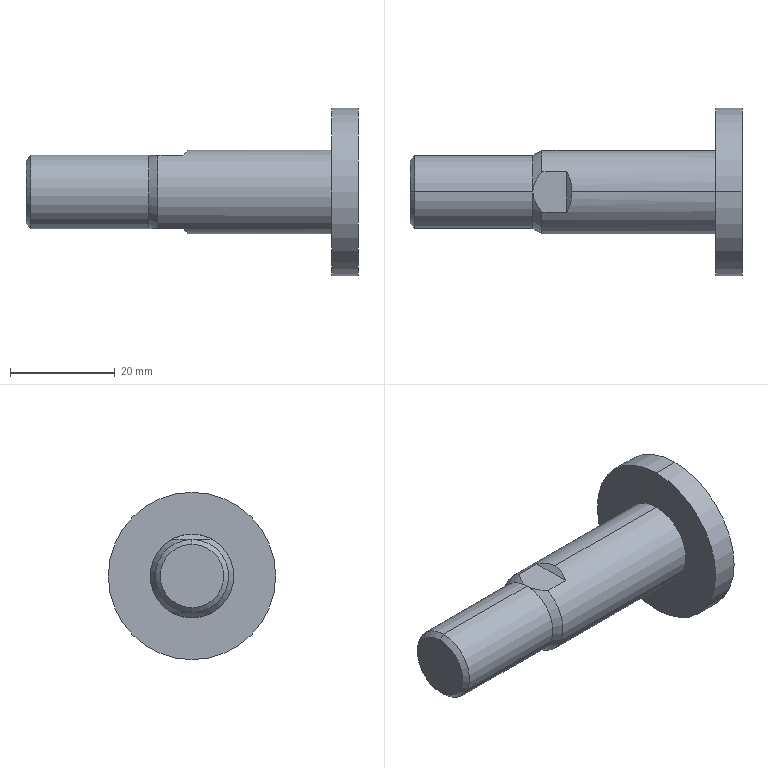Part | STEP file | SceondHI_CDQ2B32-20CMA93(0_0)_CYROD_Default | 1 solid | 17 faces | box 63.5 x 32 x 32 mm | volume 14555 mm3 | plane 7 | cylinder 6 | cone 4 | commonest cylinder face diameters 14 x2 16 x2 32 x2
STEP:
#1=CARTESIAN_POINT('',(0.,0.,0.));
#2=DIRECTION('',(0.,0.,1.));
#3=DIRECTION('',(1.,0.,0.));
#4=AXIS2_PLACEMENT_3D('',#1,#2,#3);
#5=CARTESIAN_POINT('',(30.,0.,8.));
#6=VERTEX_POINT('',#5);
#7=CARTESIAN_POINT('',(30.,0.,-8.));
#8=VERTEX_POINT('',#7);
#9=CARTESIAN_POINT('',(30.,0.,0.));
#10=DIRECTION('',(-1.,0.,0.));
#11=DIRECTION('',(0.,0.,1.));
#12=AXIS2_PLACEMENT_3D('',#9,#10,#11);
#13=CIRCLE('',#12,8.);
#14=CARTESIAN_POINT('',(35.,0.,0.));
#15=DIRECTION('',(-1.,0.,0.));
#16=DIRECTION('',(0.,0.,1.));
#17=AXIS2_PLACEMENT_3D('',#14,#15,#16);
#18=CYLINDRICAL_SURFACE('',#17,8.);
#19=CARTESIAN_POINT('',(0.,5.));
#20=DIRECTION('',(1.,0.));
#21=VECTOR('',#20,1.);
#22=LINE('',#19,#21);
#23=(GEOMETRIC_REPRESENTATION_CONTEXT(2)PARAMETRIC_REPRESENTATION_CONTEXT()REPRESENTATION_CONTEXT('',''));
#24=DEFINITIONAL_REPRESENTATION('',(#22),#23);
#25=PCURVE('',#18,#24);
#26=CARTESIAN_POINT('',(30.,8.,0.));
#27=DIRECTION('',(1.,0.,0.));
#28=DIRECTION('',(0.,0.,-1.));
#29=AXIS2_PLACEMENT_3D('',#26,#27,#28);
#30=PLANE('',#29);
#31=CARTESIAN_POINT('',(-8.,-8.));
#32=CARTESIAN_POINT('',(-8.,5.856));
#33=CARTESIAN_POINT('',(4.,-1.072));
#34=CARTESIAN_POINT('',(16.,-8.));
#35=CARTESIAN_POINT('',(4.,-14.928));
#36=CARTESIAN_POINT('',(-8.,-21.856));
#37=CARTESIAN_POINT('',(-8.,-8.));
#38=(BOUNDED_CURVE()B_SPLINE_CURVE(2,(#31,#32,#33,#34,#35,#36,#37),.UNSPECIFIED.,.T.,.F.)B_SPLINE_CURVE_WITH_KNOTS((1,2,2,2,2,1),(-2.094,0.,2.094,4.189,6.283,8.378),.UNSPECIFIED.)CURVE()GEOMETRIC_REPRESENTATION_ITEM()RATIONAL_B_SPLINE_CURVE((1.,0.5,1.,0.5,1.,0.5,1.))REPRESENTATION_ITEM(''));
#39=(GEOMETRIC_REPRESENTATION_CONTEXT(2)PARAMETRIC_REPRESENTATION_CONTEXT()REPRESENTATION_CONTEXT('',''));
#40=DEFINITIONAL_REPRESENTATION('',(#38),#39);
#41=PCURVE('',#30,#40);
#42=SURFACE_CURVE('',#13,(#25,#41),.PCURVE_S1.);
#43=EDGE_CURVE('',#6,#8,#42,.T.);
#44=ORIENTED_EDGE('',*,*,#43,.T.);
#45=CARTESIAN_POINT('',(2.5,0.,-8.));
#46=VERTEX_POINT('',#45);
#47=CARTESIAN_POINT('',(35.,0.,-8.));
#48=DIRECTION('',(-1.,0.,0.));
#49=VECTOR('',#48,1.);
#50=LINE('',#47,#49);
#51=CARTESIAN_POINT('',(3.142,0.));
#52=DIRECTION('',(0.,1.));
#53=VECTOR('',#52,1.);
#54=LINE('',#51,#53);
#55=(GEOMETRIC_REPRESENTATION_CONTEXT(2)PARAMETRIC_REPRESENTATION_CONTEXT()REPRESENTATION_CONTEXT('',''));
#56=DEFINITIONAL_REPRESENTATION('',(#54),#55);
#57=PCURVE('',#18,#56);
#58=CARTESIAN_POINT('',(35.,0.,0.));
#59=DIRECTION('',(-1.,0.,0.));
#60=DIRECTION('',(0.,0.,1.));
#61=AXIS2_PLACEMENT_3D('',#58,#59,#60);
#62=CYLINDRICAL_SURFACE('',#61,8.);
#63=CARTESIAN_POINT('',(3.142,0.));
#64=DIRECTION('',(0.,1.));
#65=VECTOR('',#64,1.);
#66=LINE('',#63,#65);
#67=(GEOMETRIC_REPRESENTATION_CONTEXT(2)PARAMETRIC_REPRESENTATION_CONTEXT()REPRESENTATION_CONTEXT('',''));
#68=DEFINITIONAL_REPRESENTATION('',(#66),#67);
#69=PCURVE('',#62,#68);
#70=SURFACE_CURVE('',#50,(#57,#69),.PCURVE_S1.);
#71=EDGE_CURVE('',#8,#46,#70,.T.);
#72=ORIENTED_EDGE('',*,*,#71,.T.);
#73=CARTESIAN_POINT('',(1.5,3.873,-7.));
#74=VERTEX_POINT('',#73);
#75=CARTESIAN_POINT('',(2.5,0.,-8.));
#76=CARTESIAN_POINT('',(2.5,1.362,-8.));
#77=CARTESIAN_POINT('',(2.159,2.681,-7.659));
#78=CARTESIAN_POINT('',(1.5,3.873,-7.));
#79=(BOUNDED_CURVE()B_SPLINE_CURVE(3,(#75,#76,#77,#78),.UNSPECIFIED.,.F.,.F.)B_SPLINE_CURVE_WITH_KNOTS((4,4),(3.142,3.647),.PIECEWISE_BEZIER_KNOTS.)CURVE()GEOMETRIC_REPRESENTATION_ITEM()RATIONAL_B_SPLINE_CURVE((1.,0.9788,0.9788,1.))REPRESENTATION_ITEM(''));
#80=CARTESIAN_POINT('',(3.142,32.5));
#81=CARTESIAN_POINT('',(3.134,32.5));
#82=CARTESIAN_POINT('',(3.119,32.501));
#83=CARTESIAN_POINT('',(3.096,32.508));
#84=CARTESIAN_POINT('',(3.073,32.518));
#85=CARTESIAN_POINT('',(3.05,32.533));
#86=CARTESIAN_POINT('',(3.027,32.552));
#87=CARTESIAN_POINT('',(3.004,32.575));
#88=CARTESIAN_POINT('',(2.981,32.602));
#89=CARTESIAN_POINT('',(2.958,32.634));
#90=CARTESIAN_POINT('',(2.935,32.669));
#91=CARTESIAN_POINT('',(2.912,32.709));
#92=CARTESIAN_POINT('',(2.889,32.753));
#93=CARTESIAN_POINT('',(2.866,32.802));
#94=CARTESIAN_POINT('',(2.843,32.854));
#95=CARTESIAN_POINT('',(2.82,32.91));
#96=CARTESIAN_POINT('',(2.797,32.971));
#97=CARTESIAN_POINT('',(2.774,33.035));
#98=CARTESIAN_POINT('',(2.751,33.103));
#99=CARTESIAN_POINT('',(2.728,33.175));
#100=CARTESIAN_POINT('',(2.705,33.251));
#101=CARTESIAN_POINT('',(2.682,33.33));
#102=CARTESIAN_POINT('',(2.659,33.413));
#103=CARTESIAN_POINT('',(2.644,33.471));
#104=CARTESIAN_POINT('',(2.636,33.5));
#105=B_SPLINE_CURVE_WITH_KNOTS('',3,(#80,#81,#82,#83,#84,#85,#86,#87,#88,#89,#90,#91,#92,#93,#94,#95,#96,#97,#98,#99,#100,#101,#102,#103,#104),.UNSPECIFIED.,.F.,.F.,(4,1,1,1,1,1,1,1,1,1,1,1,1,1,1,1,1,1,1,1,1,1,4),(3.142,3.165,3.188,3.211,3.233,3.256,3.279,3.302,3.325,3.348,3.371,3.394,3.417,3.44,3.463,3.486,3.509,3.532,3.555,3.578,3.601,3.624,3.647),.QUASI_UNIFORM_KNOTS.);
#106=(GEOMETRIC_REPRESENTATION_CONTEXT(2)PARAMETRIC_REPRESENTATION_CONTEXT()REPRESENTATION_CONTEXT('',''));
#107=DEFINITIONAL_REPRESENTATION('',(#105),#106);
#108=PCURVE('',#18,#107);
#109=CARTESIAN_POINT('',(1.5,16.,-7.));
#110=DIRECTION('',(-0.7071,0.,-0.7071));
#111=DIRECTION('',(-0.7071,0.,0.7071));
#112=AXIS2_PLACEMENT_3D('',#109,#110,#111);
#113=PLANE('',#112);
#114=CARTESIAN_POINT('',(-1.414,-16.));
#115=CARTESIAN_POINT('',(-1.414,-14.638));
#116=CARTESIAN_POINT('',(-0.9326,-13.319));
#117=CARTESIAN_POINT('',(0.,-12.127));
#118=(BOUNDED_CURVE()B_SPLINE_CURVE(3,(#114,#115,#116,#117),.UNSPECIFIED.,.F.,.F.)B_SPLINE_CURVE_WITH_KNOTS((4,4),(3.142,3.647),.PIECEWISE_BEZIER_KNOTS.)CURVE()GEOMETRIC_REPRESENTATION_ITEM()RATIONAL_B_SPLINE_CURVE((1.,0.9788,0.9788,1.))REPRESENTATION_ITEM(''));
#119=(GEOMETRIC_REPRESENTATION_CONTEXT(2)PARAMETRIC_REPRESENTATION_CONTEXT()REPRESENTATION_CONTEXT('',''));
#120=DEFINITIONAL_REPRESENTATION('',(#118),#119);
#121=PCURVE('',#113,#120);
#122=SURFACE_CURVE('',#79,(#108,#121),.PCURVE_S1.);
#123=EDGE_CURVE('',#46,#74,#122,.T.);
#124=ORIENTED_EDGE('',*,*,#123,.T.);
#125=CARTESIAN_POINT('',(-3.268,3.873,-7.));
#126=VERTEX_POINT('',#125);
#127=CARTESIAN_POINT('',(35.,3.873,-7.));
#128=DIRECTION('',(-1.,0.,0.));
#129=VECTOR('',#128,1.);
#130=LINE('',#127,#129);
#131=CARTESIAN_POINT('',(2.636,0.));
#132=DIRECTION('',(0.,1.));
#133=VECTOR('',#132,1.);
#134=LINE('',#131,#133);
#135=(GEOMETRIC_REPRESENTATION_CONTEXT(2)PARAMETRIC_REPRESENTATION_CONTEXT()REPRESENTATION_CONTEXT('',''));
#136=DEFINITIONAL_REPRESENTATION('',(#134),#135);
#137=PCURVE('',#18,#136);
#138=CARTESIAN_POINT('',(-5.,16.,-7.));
#139=DIRECTION('',(0.,0.,-1.));
#140=DIRECTION('',(-1.,0.,0.));
#141=AXIS2_PLACEMENT_3D('',#138,#139,#140);
#142=PLANE('',#141);
#143=CARTESIAN_POINT('',(-40.,-12.127));
#144=DIRECTION('',(1.,0.));
#145=VECTOR('',#144,1.);
#146=LINE('',#143,#145);
#147=(GEOMETRIC_REPRESENTATION_CONTEXT(2)PARAMETRIC_REPRESENTATION_CONTEXT()REPRESENTATION_CONTEXT('',''));
#148=DEFINITIONAL_REPRESENTATION('',(#146),#147);
#149=PCURVE('',#142,#148);
#150=SURFACE_CURVE('',#130,(#137,#149),.PCURVE_S1.);
#151=EDGE_CURVE('',#74,#126,#150,.T.);
#152=ORIENTED_EDGE('',*,*,#151,.T.);
#153=CARTESIAN_POINT('',(-3.268,3.873,7.));
#154=VERTEX_POINT('',#153);
#155=CARTESIAN_POINT('',(-3.268,0.,0.));
#156=DIRECTION('',(1.,0.,0.));
#157=DIRECTION('',(0.,0.,1.));
#158=AXIS2_PLACEMENT_3D('',#155,#156,#157);
#159=CIRCLE('',#158,8.);
#160=CARTESIAN_POINT('',(6.283,38.268));
#161=DIRECTION('',(-1.,0.));
#162=VECTOR('',#161,1.);
#163=LINE('',#160,#162);
#164=(GEOMETRIC_REPRESENTATION_CONTEXT(2)PARAMETRIC_REPRESENTATION_CONTEXT()REPRESENTATION_CONTEXT('',''));
#165=DEFINITIONAL_REPRESENTATION('',(#163),#164);
#166=PCURVE('',#18,#165);
#167=CARTESIAN_POINT('',(-3.268,0.,0.));
#168=DIRECTION('',(1.,0.,0.));
#169=DIRECTION('',(0.,0.,-1.));
#170=AXIS2_PLACEMENT_3D('',#167,#168,#169);
#171=CONICAL_SURFACE('',#170,8.,0.5236);
#172=CARTESIAN_POINT('',(-3.142,0.));
#173=DIRECTION('',(1.,0.));
#174=VECTOR('',#173,1.);
#175=LINE('',#172,#174);
#176=(GEOMETRIC_REPRESENTATION_CONTEXT(2)PARAMETRIC_REPRESENTATION_CONTEXT()REPRESENTATION_CONTEXT('',''));
#177=DEFINITIONAL_REPRESENTATION('',(#175),#176);
#178=PCURVE('',#171,#177);
#179=SURFACE_CURVE('',#159,(#166,#178),.PCURVE_S1.);
#180=EDGE_CURVE('',#126,#154,#179,.T.);
#181=ORIENTED_EDGE('',*,*,#180,.T.);
#182=CARTESIAN_POINT('',(1.5,3.873,7.));
#183=VERTEX_POINT('',#182);
#184=CARTESIAN_POINT('',(35.,3.873,7.));
#185=DIRECTION('',(1.,0.,0.));
#186=VECTOR('',#185,1.);
#187=LINE('',#184,#186);
#188=CARTESIAN_POINT('',(0.5054,0.));
#189=DIRECTION('',(0.,-1.));
#190=VECTOR('',#189,1.);
#191=LINE('',#188,#190);
#192=(GEOMETRIC_REPRESENTATION_CONTEXT(2)PARAMETRIC_REPRESENTATION_CONTEXT()REPRESENTATION_CONTEXT('',''));
#193=DEFINITIONAL_REPRESENTATION('',(#191),#192);
#194=PCURVE('',#18,#193);
#195=CARTESIAN_POINT('',(1.5,16.,7.));
#196=DIRECTION('',(0.,0.,1.));
#197=DIRECTION('',(1.,0.,0.));
#198=AXIS2_PLACEMENT_3D('',#195,#196,#197);
#199=PLANE('',#198);
#200=CARTESIAN_POINT('',(33.5,-12.127));
#201=DIRECTION('',(1.,0.));
#202=VECTOR('',#201,1.);
#203=LINE('',#200,#202);
#204=(GEOMETRIC_REPRESENTATION_CONTEXT(2)PARAMETRIC_REPRESENTATION_CONTEXT()REPRESENTATION_CONTEXT('',''));
#205=DEFINITIONAL_REPRESENTATION('',(#203),#204);
#206=PCURVE('',#199,#205);
#207=SURFACE_CURVE('',#187,(#194,#206),.PCURVE_S1.);
#208=EDGE_CURVE('',#154,#183,#207,.T.);
#209=ORIENTED_EDGE('',*,*,#208,.T.);
#210=CARTESIAN_POINT('',(2.5,0.,8.));
#211=VERTEX_POINT('',#210);
#212=CARTESIAN_POINT('',(1.5,3.873,7.));
#213=CARTESIAN_POINT('',(2.159,2.681,7.659));
#214=CARTESIAN_POINT('',(2.5,1.362,8.));
#215=CARTESIAN_POINT('',(2.5,0.,8.));
#216=(BOUNDED_CURVE()B_SPLINE_CURVE(3,(#212,#213,#214,#215),.UNSPECIFIED.,.F.,.F.)B_SPLINE_CURVE_WITH_KNOTS((4,4),(2.636,3.142),.PIECEWISE_BEZIER_KNOTS.)CURVE()GEOMETRIC_REPRESENTATION_ITEM()RATIONAL_B_SPLINE_CURVE((1.,0.9788,0.9788,1.))REPRESENTATION_ITEM(''));
#217=CARTESIAN_POINT('',(0.5054,33.5));
#218=CARTESIAN_POINT('',(0.4978,33.471));
#219=CARTESIAN_POINT('',(0.4826,33.413));
#220=CARTESIAN_POINT('',(0.4598,33.33));
#221=CARTESIAN_POINT('',(0.4369,33.251));
#222=CARTESIAN_POINT('',(0.414,33.175));
#223=CARTESIAN_POINT('',(0.391,33.103));
#224=CARTESIAN_POINT('',(0.368,33.035));
#225=CARTESIAN_POINT('',(0.345,32.971));
#226=CARTESIAN_POINT('',(0.3219,32.91));
#227=CARTESIAN_POINT('',(0.2989,32.854));
#228=CARTESIAN_POINT('',(0.2758,32.802));
#229=CARTESIAN_POINT('',(0.2527,32.753));
#230=CARTESIAN_POINT('',(0.2296,32.709));
#231=CARTESIAN_POINT('',(0.2065,32.669));
#232=CARTESIAN_POINT('',(0.1834,32.634));
#233=CARTESIAN_POINT('',(0.1604,32.602));
#234=CARTESIAN_POINT('',(0.1373,32.575));
#235=CARTESIAN_POINT('',(0.1143,32.552));
#236=CARTESIAN_POINT('',(0.09137,32.533));
#237=CARTESIAN_POINT('',(0.06844,32.518));
#238=CARTESIAN_POINT('',(0.04557,32.508));
#239=CARTESIAN_POINT('',(0.02275,32.501));
#240=CARTESIAN_POINT('',(0.007576,32.5));
#241=CARTESIAN_POINT('',(0.,32.5));
#242=B_SPLINE_CURVE_WITH_KNOTS('',3,(#217,#218,#219,#220,#221,#222,#223,#224,#225,#226,#227,#228,#229,#230,#231,#232,#233,#234,#235,#236,#237,#238,#239,#240,#241),.UNSPECIFIED.,.F.,.F.,(4,1,1,1,1,1,1,1,1,1,1,1,1,1,1,1,1,1,1,1,1,1,4),(2.636,2.659,2.682,2.705,2.728,2.751,2.774,2.797,2.82,2.843,2.866,2.889,2.912,2.935,2.958,2.981,3.004,3.027,3.05,3.073,3.096,3.119,3.142),.QUASI_UNIFORM_KNOTS.);
#243=(GEOMETRIC_REPRESENTATION_CONTEXT(2)PARAMETRIC_REPRESENTATION_CONTEXT()REPRESENTATION_CONTEXT('',''));
#244=DEFINITIONAL_REPRESENTATION('',(#242),#243);
#245=PCURVE('',#18,#244);
#246=CARTESIAN_POINT('',(6.5,16.,12.));
#247=DIRECTION('',(-0.7071,0.,0.7071));
#248=DIRECTION('',(0.7071,0.,0.7071));
#249=AXIS2_PLACEMENT_3D('',#246,#247,#248);
#250=PLANE('',#249);
#251=CARTESIAN_POINT('',(-7.071,-12.127));
#252=CARTESIAN_POINT('',(-6.138,-13.319));
#253=CARTESIAN_POINT('',(-5.657,-14.638));
#254=CARTESIAN_POINT('',(-5.657,-16.));
#255=(BOUNDED_CURVE()B_SPLINE_CURVE(3,(#251,#252,#253,#254),.UNSPECIFIED.,.F.,.F.)B_SPLINE_CURVE_WITH_KNOTS((4,4),(2.636,3.142),.PIECEWISE_BEZIER_KNOTS.)CURVE()GEOMETRIC_REPRESENTATION_ITEM()RATIONAL_B_SPLINE_CURVE((1.,0.9788,0.9788,1.))REPRESENTATION_ITEM(''));
#256=(GEOMETRIC_REPRESENTATION_CONTEXT(2)PARAMETRIC_REPRESENTATION_CONTEXT()REPRESENTATION_CONTEXT('',''));
#257=DEFINITIONAL_REPRESENTATION('',(#255),#256);
#258=PCURVE('',#250,#257);
#259=SURFACE_CURVE('',#216,(#245,#258),.PCURVE_S1.);
#260=EDGE_CURVE('',#183,#211,#259,.T.);
#261=ORIENTED_EDGE('',*,*,#260,.T.);
#262=CARTESIAN_POINT('',(35.,0.,8.));
#263=DIRECTION('',(-1.,0.,0.));
#264=VECTOR('',#263,1.);
#265=LINE('',#262,#264);
#266=CARTESIAN_POINT('',(0.,0.));
#267=DIRECTION('',(0.,1.));
#268=VECTOR('',#267,1.);
#269=LINE('',#266,#268);
#270=(GEOMETRIC_REPRESENTATION_CONTEXT(2)PARAMETRIC_REPRESENTATION_CONTEXT()REPRESENTATION_CONTEXT('',''));
#271=DEFINITIONAL_REPRESENTATION('',(#269),#270);
#272=PCURVE('',#18,#271);
#273=CARTESIAN_POINT('',(6.283,0.));
#274=DIRECTION('',(0.,1.));
#275=VECTOR('',#274,1.);
#276=LINE('',#273,#275);
#277=(GEOMETRIC_REPRESENTATION_CONTEXT(2)PARAMETRIC_REPRESENTATION_CONTEXT()REPRESENTATION_CONTEXT('',''));
#278=DEFINITIONAL_REPRESENTATION('',(#276),#277);
#279=PCURVE('',#62,#278);
#280=SURFACE_CURVE('',#265,(#272,#279),.PCURVE_S1.);
#281=EDGE_CURVE('',#6,#211,#280,.T.);
#282=ORIENTED_EDGE('',*,*,#281,.F.);
#283=EDGE_LOOP('',(#44,#72,#124,#152,#181,#209,#261,#282));
#284=FACE_BOUND('',#283,.T.);
#285=ADVANCED_FACE('',(#284),#18,.T.);
#286=CARTESIAN_POINT('',(-5.,0.,-7.));
#287=VERTEX_POINT('',#286);
#288=CARTESIAN_POINT('',(-5.,0.,7.));
#289=VERTEX_POINT('',#288);
#290=CARTESIAN_POINT('',(-5.,0.,0.));
#291=DIRECTION('',(1.,0.,0.));
#292=DIRECTION('',(0.,0.,-1.));
#293=AXIS2_PLACEMENT_3D('',#290,#291,#292);
#294=CIRCLE('',#293,7.);
#295=CARTESIAN_POINT('',(35.,0.,0.));
#296=DIRECTION('',(-1.,0.,0.));
#297=DIRECTION('',(0.,0.,1.));
#298=AXIS2_PLACEMENT_3D('',#295,#296,#297);
#299=CYLINDRICAL_SURFACE('',#298,7.);
#300=CARTESIAN_POINT('',(3.142,40.));
#301=DIRECTION('',(-1.,0.));
#302=VECTOR('',#301,1.);
#303=LINE('',#300,#302);
#304=(GEOMETRIC_REPRESENTATION_CONTEXT(2)PARAMETRIC_REPRESENTATION_CONTEXT()REPRESENTATION_CONTEXT('',''));
#305=DEFINITIONAL_REPRESENTATION('',(#303),#304);
#306=PCURVE('',#299,#305);
#307=CARTESIAN_POINT('',(0.,-1.732));
#308=DIRECTION('',(1.,0.));
#309=VECTOR('',#308,1.);
#310=LINE('',#307,#309);
#311=(GEOMETRIC_REPRESENTATION_CONTEXT(2)PARAMETRIC_REPRESENTATION_CONTEXT()REPRESENTATION_CONTEXT('',''));
#312=DEFINITIONAL_REPRESENTATION('',(#310),#311);
#313=PCURVE('',#171,#312);
#314=SURFACE_CURVE('',#294,(#306,#313),.PCURVE_S1.);
#315=EDGE_CURVE('',#287,#289,#314,.T.);
#316=ORIENTED_EDGE('',*,*,#315,.F.);
#317=CARTESIAN_POINT('',(-27.58,0.,-7.));
#318=VERTEX_POINT('',#317);
#319=CARTESIAN_POINT('',(35.,0.,-7.));
#320=DIRECTION('',(-1.,0.,0.));
#321=VECTOR('',#320,1.);
#322=LINE('',#319,#321);
#323=CARTESIAN_POINT('',(3.142,0.));
#324=DIRECTION('',(0.,1.));
#325=VECTOR('',#324,1.);
#326=LINE('',#323,#325);
#327=(GEOMETRIC_REPRESENTATION_CONTEXT(2)PARAMETRIC_REPRESENTATION_CONTEXT()REPRESENTATION_CONTEXT('',''));
#328=DEFINITIONAL_REPRESENTATION('',(#326),#327);
#329=PCURVE('',#299,#328);
#330=CARTESIAN_POINT('',(35.,0.,0.));
#331=DIRECTION('',(-1.,0.,0.));
#332=DIRECTION('',(0.,0.,1.));
#333=AXIS2_PLACEMENT_3D('',#330,#331,#332);
#334=CYLINDRICAL_SURFACE('',#333,7.);
#335=CARTESIAN_POINT('',(3.142,0.));
#336=DIRECTION('',(0.,1.));
#337=VECTOR('',#336,1.);
#338=LINE('',#335,#337);
#339=(GEOMETRIC_REPRESENTATION_CONTEXT(2)PARAMETRIC_REPRESENTATION_CONTEXT()REPRESENTATION_CONTEXT('',''));
#340=DEFINITIONAL_REPRESENTATION('',(#338),#339);
#341=PCURVE('',#334,#340);
#342=SURFACE_CURVE('',#322,(#329,#341),.PCURVE_S1.);
#343=EDGE_CURVE('',#287,#318,#342,.T.);
#344=ORIENTED_EDGE('',*,*,#343,.T.);
#345=CARTESIAN_POINT('',(-27.58,0.,7.));
#346=VERTEX_POINT('',#345);
#347=CARTESIAN_POINT('',(-27.58,0.,0.));
#348=DIRECTION('',(1.,0.,0.));
#349=DIRECTION('',(0.,0.,1.));
#350=AXIS2_PLACEMENT_3D('',#347,#348,#349);
#351=CIRCLE('',#350,7.);
#352=CARTESIAN_POINT('',(6.283,62.58));
#353=DIRECTION('',(-1.,0.));
#354=VECTOR('',#353,1.);
#355=LINE('',#352,#354);
#356=(GEOMETRIC_REPRESENTATION_CONTEXT(2)PARAMETRIC_REPRESENTATION_CONTEXT()REPRESENTATION_CONTEXT('',''));
#357=DEFINITIONAL_REPRESENTATION('',(#355),#356);
#358=PCURVE('',#299,#357);
#359=CARTESIAN_POINT('',(-27.58,0.,0.));
#360=DIRECTION('',(1.,0.,0.));
#361=DIRECTION('',(0.,0.,-1.));
#362=AXIS2_PLACEMENT_3D('',#359,#360,#361);
#363=CONICAL_SURFACE('',#362,7.,0.7854);
#364=CARTESIAN_POINT('',(-3.142,0.));
#365=DIRECTION('',(1.,0.));
#366=VECTOR('',#365,1.);
#367=LINE('',#364,#366);
#368=(GEOMETRIC_REPRESENTATION_CONTEXT(2)PARAMETRIC_REPRESENTATION_CONTEXT()REPRESENTATION_CONTEXT('',''));
#369=DEFINITIONAL_REPRESENTATION('',(#367),#368);
#370=PCURVE('',#363,#369);
#371=SURFACE_CURVE('',#351,(#358,#370),.PCURVE_S1.);
#372=EDGE_CURVE('',#318,#346,#371,.T.);
#373=ORIENTED_EDGE('',*,*,#372,.T.);
#374=CARTESIAN_POINT('',(35.,0.,7.));
#375=DIRECTION('',(-1.,0.,0.));
#376=VECTOR('',#375,1.);
#377=LINE('',#374,#376);
#378=CARTESIAN_POINT('',(0.,0.));
#379=DIRECTION('',(0.,1.));
#380=VECTOR('',#379,1.);
#381=LINE('',#378,#380);
#382=(GEOMETRIC_REPRESENTATION_CONTEXT(2)PARAMETRIC_REPRESENTATION_CONTEXT()REPRESENTATION_CONTEXT('',''));
#383=DEFINITIONAL_REPRESENTATION('',(#381),#382);
#384=PCURVE('',#299,#383);
#385=CARTESIAN_POINT('',(6.283,0.));
#386=DIRECTION('',(0.,1.));
#387=VECTOR('',#386,1.);
#388=LINE('',#385,#387);
#389=(GEOMETRIC_REPRESENTATION_CONTEXT(2)PARAMETRIC_REPRESENTATION_CONTEXT()REPRESENTATION_CONTEXT('',''));
#390=DEFINITIONAL_REPRESENTATION('',(#388),#389);
#391=PCURVE('',#334,#390);
#392=SURFACE_CURVE('',#377,(#384,#391),.PCURVE_S1.);
#393=EDGE_CURVE('',#289,#346,#392,.T.);
#394=ORIENTED_EDGE('',*,*,#393,.F.);
#395=EDGE_LOOP('',(#316,#344,#373,#394));
#396=FACE_BOUND('',#395,.T.);
#397=ADVANCED_FACE('',(#396),#299,.T.);
#398=CARTESIAN_POINT('',(35.,0.,16.));
#399=VERTEX_POINT('',#398);
#400=CARTESIAN_POINT('',(35.,0.,-16.));
#401=VERTEX_POINT('',#400);
#402=CARTESIAN_POINT('',(35.,0.,0.));
#403=DIRECTION('',(-1.,0.,0.));
#404=DIRECTION('',(0.,0.,1.));
#405=AXIS2_PLACEMENT_3D('',#402,#403,#404);
#406=CIRCLE('',#405,16.);
#407=CARTESIAN_POINT('',(35.,0.,0.));
#408=DIRECTION('',(-1.,0.,0.));
#409=DIRECTION('',(0.,0.,1.));
#410=AXIS2_PLACEMENT_3D('',#407,#408,#409);
#411=CYLINDRICAL_SURFACE('',#410,16.);
#412=CARTESIAN_POINT('',(0.,0.));
#413=DIRECTION('',(1.,0.));
#414=VECTOR('',#413,1.);
#415=LINE('',#412,#414);
#416=(GEOMETRIC_REPRESENTATION_CONTEXT(2)PARAMETRIC_REPRESENTATION_CONTEXT()REPRESENTATION_CONTEXT('',''));
#417=DEFINITIONAL_REPRESENTATION('',(#415),#416);
#418=PCURVE('',#411,#417);
#419=CARTESIAN_POINT('',(35.,16.,0.));
#420=DIRECTION('',(-1.,0.,0.));
#421=DIRECTION('',(0.,0.,1.));
#422=AXIS2_PLACEMENT_3D('',#419,#420,#421);
#423=PLANE('',#422);
#424=CARTESIAN_POINT('',(0.,-16.));
#425=DIRECTION('',(1.,0.));
#426=AXIS2_PLACEMENT_2D('',#424,#425);
#427=CIRCLE('',#426,16.);
#428=(GEOMETRIC_REPRESENTATION_CONTEXT(2)PARAMETRIC_REPRESENTATION_CONTEXT()REPRESENTATION_CONTEXT('',''));
#429=DEFINITIONAL_REPRESENTATION('',(#427),#428);
#430=PCURVE('',#423,#429);
#431=SURFACE_CURVE('',#406,(#418,#430),.PCURVE_S1.);
#432=EDGE_CURVE('',#399,#401,#431,.T.);
#433=ORIENTED_EDGE('',*,*,#432,.T.);
#434=CARTESIAN_POINT('',(30.,0.,-16.));
#435=VERTEX_POINT('',#434);
#436=CARTESIAN_POINT('',(35.,0.,-16.));
#437=DIRECTION('',(-1.,0.,0.));
#438=VECTOR('',#437,1.);
#439=LINE('',#436,#438);
#440=CARTESIAN_POINT('',(3.142,0.));
#441=DIRECTION('',(0.,1.));
#442=VECTOR('',#441,1.);
#443=LINE('',#440,#442);
#444=(GEOMETRIC_REPRESENTATION_CONTEXT(2)PARAMETRIC_REPRESENTATION_CONTEXT()REPRESENTATION_CONTEXT('',''));
#445=DEFINITIONAL_REPRESENTATION('',(#443),#444);
#446=PCURVE('',#411,#445);
#447=CARTESIAN_POINT('',(35.,0.,0.));
#448=DIRECTION('',(-1.,0.,0.));
#449=DIRECTION('',(0.,0.,1.));
#450=AXIS2_PLACEMENT_3D('',#447,#448,#449);
#451=CYLINDRICAL_SURFACE('',#450,16.);
#452=CARTESIAN_POINT('',(3.142,0.));
#453=DIRECTION('',(0.,1.));
#454=VECTOR('',#453,1.);
#455=LINE('',#452,#454);
#456=(GEOMETRIC_REPRESENTATION_CONTEXT(2)PARAMETRIC_REPRESENTATION_CONTEXT()REPRESENTATION_CONTEXT('',''));
#457=DEFINITIONAL_REPRESENTATION('',(#455),#456);
#458=PCURVE('',#451,#457);
#459=SURFACE_CURVE('',#439,(#446,#458),.PCURVE_S1.);
#460=EDGE_CURVE('',#401,#435,#459,.T.);
#461=ORIENTED_EDGE('',*,*,#460,.T.);
#462=CARTESIAN_POINT('',(30.,0.,16.));
#463=VERTEX_POINT('',#462);
#464=CARTESIAN_POINT('',(30.,0.,0.));
#465=DIRECTION('',(1.,0.,0.));
#466=DIRECTION('',(0.,0.,1.));
#467=AXIS2_PLACEMENT_3D('',#464,#465,#466);
#468=CIRCLE('',#467,16.);
#469=CARTESIAN_POINT('',(6.283,5.));
#470=DIRECTION('',(-1.,0.));
#471=VECTOR('',#470,1.);
#472=LINE('',#469,#471);
#473=(GEOMETRIC_REPRESENTATION_CONTEXT(2)PARAMETRIC_REPRESENTATION_CONTEXT()REPRESENTATION_CONTEXT('',''));
#474=DEFINITIONAL_REPRESENTATION('',(#472),#473);
#475=PCURVE('',#411,#474);
#476=CARTESIAN_POINT('',(0.,-8.));
#477=DIRECTION('',(-1.,0.));
#478=AXIS2_PLACEMENT_2D('',#476,#477);
#479=CIRCLE('',#478,16.);
#480=(GEOMETRIC_REPRESENTATION_CONTEXT(2)PARAMETRIC_REPRESENTATION_CONTEXT()REPRESENTATION_CONTEXT('',''));
#481=DEFINITIONAL_REPRESENTATION('',(#479),#480);
#482=PCURVE('',#30,#481);
#483=SURFACE_CURVE('',#468,(#475,#482),.PCURVE_S1.);
#484=EDGE_CURVE('',#435,#463,#483,.T.);
#485=ORIENTED_EDGE('',*,*,#484,.T.);
#486=CARTESIAN_POINT('',(35.,0.,16.));
#487=DIRECTION('',(-1.,0.,0.));
#488=VECTOR('',#487,1.);
#489=LINE('',#486,#488);
#490=CARTESIAN_POINT('',(0.,0.));
#491=DIRECTION('',(0.,1.));
#492=VECTOR('',#491,1.);
#493=LINE('',#490,#492);
#494=(GEOMETRIC_REPRESENTATION_CONTEXT(2)PARAMETRIC_REPRESENTATION_CONTEXT()REPRESENTATION_CONTEXT('',''));
#495=DEFINITIONAL_REPRESENTATION('',(#493),#494);
#496=PCURVE('',#411,#495);
#497=CARTESIAN_POINT('',(6.283,0.));
#498=DIRECTION('',(0.,1.));
#499=VECTOR('',#498,1.);
#500=LINE('',#497,#499);
#501=(GEOMETRIC_REPRESENTATION_CONTEXT(2)PARAMETRIC_REPRESENTATION_CONTEXT()REPRESENTATION_CONTEXT('',''));
#502=DEFINITIONAL_REPRESENTATION('',(#500),#501);
#503=PCURVE('',#451,#502);
#504=SURFACE_CURVE('',#489,(#496,#503),.PCURVE_S1.);
#505=EDGE_CURVE('',#399,#463,#504,.T.);
#506=ORIENTED_EDGE('',*,*,#505,.F.);
#507=EDGE_LOOP('',(#433,#461,#485,#506));
#508=FACE_BOUND('',#507,.T.);
#509=ADVANCED_FACE('',(#508),#411,.T.);
#510=CARTESIAN_POINT('',(-28.5,0.,-6.08));
#511=VERTEX_POINT('',#510);
#512=CARTESIAN_POINT('',(-28.5,0.,6.08));
#513=VERTEX_POINT('',#512);
#514=CARTESIAN_POINT('',(-28.5,0.,0.));
#515=DIRECTION('',(1.,0.,0.));
#516=DIRECTION('',(0.,0.,-1.));
#517=AXIS2_PLACEMENT_3D('',#514,#515,#516);
#518=CIRCLE('',#517,6.08);
#519=CARTESIAN_POINT('',(0.,-0.92));
#520=DIRECTION('',(1.,0.));
#521=VECTOR('',#520,1.);
#522=LINE('',#519,#521);
#523=(GEOMETRIC_REPRESENTATION_CONTEXT(2)PARAMETRIC_REPRESENTATION_CONTEXT()REPRESENTATION_CONTEXT('',''));
#524=DEFINITIONAL_REPRESENTATION('',(#522),#523);
#525=PCURVE('',#363,#524);
#526=CARTESIAN_POINT('',(-28.5,0.,0.));
#527=DIRECTION('',(1.,0.,0.));
#528=DIRECTION('',(0.,0.,-1.));
#529=AXIS2_PLACEMENT_3D('',#526,#527,#528);
#530=PLANE('',#529);
#531=CARTESIAN_POINT('',(0.,0.));
#532=DIRECTION('',(1.,0.));
#533=AXIS2_PLACEMENT_2D('',#531,#532);
#534=CIRCLE('',#533,6.08);
#535=(GEOMETRIC_REPRESENTATION_CONTEXT(2)PARAMETRIC_REPRESENTATION_CONTEXT()REPRESENTATION_CONTEXT('',''));
#536=DEFINITIONAL_REPRESENTATION('',(#534),#535);
#537=PCURVE('',#530,#536);
#538=SURFACE_CURVE('',#518,(#525,#537),.PCURVE_S1.);
#539=EDGE_CURVE('',#511,#513,#538,.T.);
#540=ORIENTED_EDGE('',*,*,#539,.T.);
#541=CARTESIAN_POINT('',(-27.58,0.,7.));
#542=DIRECTION('',(0.7071,0.,0.7071));
#543=VECTOR('',#542,1.);
#544=LINE('',#541,#543);
#545=CARTESIAN_POINT('',(3.142,0.));
#546=DIRECTION('',(0.,1.));
#547=VECTOR('',#546,1.);
#548=LINE('',#545,#547);
#549=(GEOMETRIC_REPRESENTATION_CONTEXT(2)PARAMETRIC_REPRESENTATION_CONTEXT()REPRESENTATION_CONTEXT('',''));
#550=DEFINITIONAL_REPRESENTATION('',(#548),#549);
#551=PCURVE('',#363,#550);
#552=CARTESIAN_POINT('',(-27.58,0.,0.));
#553=DIRECTION('',(1.,0.,0.));
#554=DIRECTION('',(0.,0.,-1.));
#555=AXIS2_PLACEMENT_3D('',#552,#553,#554);
#556=CONICAL_SURFACE('',#555,7.,0.7854);
#557=CARTESIAN_POINT('',(3.142,0.));
#558=DIRECTION('',(0.,1.));
#559=VECTOR('',#558,1.);
#560=LINE('',#557,#559);
#561=(GEOMETRIC_REPRESENTATION_CONTEXT(2)PARAMETRIC_REPRESENTATION_CONTEXT()REPRESENTATION_CONTEXT('',''));
#562=DEFINITIONAL_REPRESENTATION('',(#560),#561);
#563=PCURVE('',#556,#562);
#564=SURFACE_CURVE('',#544,(#551,#563),.PCURVE_S1.);
#565=EDGE_CURVE('',#513,#346,#564,.T.);
#566=ORIENTED_EDGE('',*,*,#565,.T.);
#567=ORIENTED_EDGE('',*,*,#372,.F.);
#568=CARTESIAN_POINT('',(-27.58,0.,-7.));
#569=DIRECTION('',(0.7071,0.,-0.7071));
#570=VECTOR('',#569,1.);
#571=LINE('',#568,#570);
#572=CARTESIAN_POINT('',(0.,0.));
#573=DIRECTION('',(0.,1.));
#574=VECTOR('',#573,1.);
#575=LINE('',#572,#574);
#576=(GEOMETRIC_REPRESENTATION_CONTEXT(2)PARAMETRIC_REPRESENTATION_CONTEXT()REPRESENTATION_CONTEXT('',''));
#577=DEFINITIONAL_REPRESENTATION('',(#575),#576);
#578=PCURVE('',#363,#577);
#579=CARTESIAN_POINT('',(6.283,0.));
#580=DIRECTION('',(0.,1.));
#581=VECTOR('',#580,1.);
#582=LINE('',#579,#581);
#583=(GEOMETRIC_REPRESENTATION_CONTEXT(2)PARAMETRIC_REPRESENTATION_CONTEXT()REPRESENTATION_CONTEXT('',''));
#584=DEFINITIONAL_REPRESENTATION('',(#582),#583);
#585=PCURVE('',#556,#584);
#586=SURFACE_CURVE('',#571,(#578,#585),.PCURVE_S1.);
#587=EDGE_CURVE('',#511,#318,#586,.T.);
#588=ORIENTED_EDGE('',*,*,#587,.F.);
#589=EDGE_LOOP('',(#540,#566,#567,#588));
#590=FACE_BOUND('',#589,.T.);
#591=ADVANCED_FACE('',(#590),#363,.T.);
#592=ORIENTED_EDGE('',*,*,#71,.F.);
#593=CARTESIAN_POINT('',(30.,0.,0.));
#594=DIRECTION('',(-1.,0.,0.));
#595=DIRECTION('',(0.,0.,1.));
#596=AXIS2_PLACEMENT_3D('',#593,#594,#595);
#597=CIRCLE('',#596,8.);
#598=CARTESIAN_POINT('',(0.,5.));
#599=DIRECTION('',(1.,0.));
#600=VECTOR('',#599,1.);
#601=LINE('',#598,#600);
#602=(GEOMETRIC_REPRESENTATION_CONTEXT(2)PARAMETRIC_REPRESENTATION_CONTEXT()REPRESENTATION_CONTEXT('',''));
#603=DEFINITIONAL_REPRESENTATION('',(#601),#602);
#604=PCURVE('',#62,#603);
#605=CARTESIAN_POINT('',(-8.,-8.));
#606=CARTESIAN_POINT('',(-8.,5.856));
#607=CARTESIAN_POINT('',(4.,-1.072));
#608=CARTESIAN_POINT('',(16.,-8.));
#609=CARTESIAN_POINT('',(4.,-14.928));
#610=CARTESIAN_POINT('',(-8.,-21.856));
#611=CARTESIAN_POINT('',(-8.,-8.));
#612=(BOUNDED_CURVE()B_SPLINE_CURVE(2,(#605,#606,#607,#608,#609,#610,#611),.UNSPECIFIED.,.T.,.F.)B_SPLINE_CURVE_WITH_KNOTS((1,2,2,2,2,1),(-2.094,0.,2.094,4.189,6.283,8.378),.UNSPECIFIED.)CURVE()GEOMETRIC_REPRESENTATION_ITEM()RATIONAL_B_SPLINE_CURVE((1.,0.5,1.,0.5,1.,0.5,1.))REPRESENTATION_ITEM(''));
#613=(GEOMETRIC_REPRESENTATION_CONTEXT(2)PARAMETRIC_REPRESENTATION_CONTEXT()REPRESENTATION_CONTEXT('',''));
#614=DEFINITIONAL_REPRESENTATION('',(#612),#613);
#615=PCURVE('',#30,#614);
#616=SURFACE_CURVE('',#597,(#604,#615),.PCURVE_S1.);
#617=EDGE_CURVE('',#8,#6,#616,.T.);
#618=ORIENTED_EDGE('',*,*,#617,.T.);
#619=ORIENTED_EDGE('',*,*,#281,.T.);
#620=CARTESIAN_POINT('',(1.5,-3.873,7.));
#621=VERTEX_POINT('',#620);
#622=CARTESIAN_POINT('',(2.5,0.,8.));
#623=CARTESIAN_POINT('',(2.5,-1.362,8.));
#624=CARTESIAN_POINT('',(2.159,-2.681,7.659));
#625=CARTESIAN_POINT('',(1.5,-3.873,7.));
#626=(BOUNDED_CURVE()B_SPLINE_CURVE(3,(#622,#623,#624,#625),.UNSPECIFIED.,.F.,.F.)B_SPLINE_CURVE_WITH_KNOTS((4,4),(3.142,3.647),.PIECEWISE_BEZIER_KNOTS.)CURVE()GEOMETRIC_REPRESENTATION_ITEM()RATIONAL_B_SPLINE_CURVE((1.,0.9788,0.9788,1.))REPRESENTATION_ITEM(''));
#627=CARTESIAN_POINT('',(6.283,32.5));
#628=CARTESIAN_POINT('',(6.276,32.5));
#629=CARTESIAN_POINT('',(6.26,32.501));
#630=CARTESIAN_POINT('',(6.238,32.508));
#631=CARTESIAN_POINT('',(6.215,32.518));
#632=CARTESIAN_POINT('',(6.192,32.533));
#633=CARTESIAN_POINT('',(6.169,32.552));
#634=CARTESIAN_POINT('',(6.146,32.575));
#635=CARTESIAN_POINT('',(6.123,32.602));
#636=CARTESIAN_POINT('',(6.1,32.634));
#637=CARTESIAN_POINT('',(6.077,32.669));
#638=CARTESIAN_POINT('',(6.054,32.709));
#639=CARTESIAN_POINT('',(6.031,32.753));
#640=CARTESIAN_POINT('',(6.007,32.802));
#641=CARTESIAN_POINT('',(5.984,32.854));
#642=CARTESIAN_POINT('',(5.961,32.91));
#643=CARTESIAN_POINT('',(5.938,32.971));
#644=CARTESIAN_POINT('',(5.915,33.035));
#645=CARTESIAN_POINT('',(5.892,33.103));
#646=CARTESIAN_POINT('',(5.869,33.175));
#647=CARTESIAN_POINT('',(5.846,33.251));
#648=CARTESIAN_POINT('',(5.823,33.33));
#649=CARTESIAN_POINT('',(5.801,33.413));
#650=CARTESIAN_POINT('',(5.785,33.471));
#651=CARTESIAN_POINT('',(5.778,33.5));
#652=B_SPLINE_CURVE_WITH_KNOTS('',3,(#627,#628,#629,#630,#631,#632,#633,#634,#635,#636,#637,#638,#639,#640,#641,#642,#643,#644,#645,#646,#647,#648,#649,#650,#651),.UNSPECIFIED.,.F.,.F.,(4,1,1,1,1,1,1,1,1,1,1,1,1,1,1,1,1,1,1,1,1,1,4),(3.142,3.165,3.188,3.211,3.233,3.256,3.279,3.302,3.325,3.348,3.371,3.394,3.417,3.44,3.463,3.486,3.509,3.532,3.555,3.578,3.601,3.624,3.647),.QUASI_UNIFORM_KNOTS.);
#653=(GEOMETRIC_REPRESENTATION_CONTEXT(2)PARAMETRIC_REPRESENTATION_CONTEXT()REPRESENTATION_CONTEXT('',''));
#654=DEFINITIONAL_REPRESENTATION('',(#652),#653);
#655=PCURVE('',#62,#654);
#656=CARTESIAN_POINT('',(-5.657,-16.));
#657=CARTESIAN_POINT('',(-5.657,-17.362));
#658=CARTESIAN_POINT('',(-6.138,-18.681));
#659=CARTESIAN_POINT('',(-7.071,-19.873));
#660=(BOUNDED_CURVE()B_SPLINE_CURVE(3,(#656,#657,#658,#659),.UNSPECIFIED.,.F.,.F.)B_SPLINE_CURVE_WITH_KNOTS((4,4),(3.142,3.647),.PIECEWISE_BEZIER_KNOTS.)CURVE()GEOMETRIC_REPRESENTATION_ITEM()RATIONAL_B_SPLINE_CURVE((1.,0.9788,0.9788,1.))REPRESENTATION_ITEM(''));
#661=(GEOMETRIC_REPRESENTATION_CONTEXT(2)PARAMETRIC_REPRESENTATION_CONTEXT()REPRESENTATION_CONTEXT('',''));
#662=DEFINITIONAL_REPRESENTATION('',(#660),#661);
#663=PCURVE('',#250,#662);
#664=SURFACE_CURVE('',#626,(#655,#663),.PCURVE_S1.);
#665=EDGE_CURVE('',#211,#621,#664,.T.);
#666=ORIENTED_EDGE('',*,*,#665,.T.);
#667=CARTESIAN_POINT('',(-3.268,-3.873,7.));
#668=VERTEX_POINT('',#667);
#669=CARTESIAN_POINT('',(35.,-3.873,7.));
#670=DIRECTION('',(-1.,0.,0.));
#671=VECTOR('',#670,1.);
#672=LINE('',#669,#671);
#673=CARTESIAN_POINT('',(5.778,0.));
#674=DIRECTION('',(0.,1.));
#675=VECTOR('',#674,1.);
#676=LINE('',#673,#675);
#677=(GEOMETRIC_REPRESENTATION_CONTEXT(2)PARAMETRIC_REPRESENTATION_CONTEXT()REPRESENTATION_CONTEXT('',''));
#678=DEFINITIONAL_REPRESENTATION('',(#676),#677);
#679=PCURVE('',#62,#678);
#680=CARTESIAN_POINT('',(33.5,-19.873));
#681=DIRECTION('',(-1.,0.));
#682=VECTOR('',#681,1.);
#683=LINE('',#680,#682);
#684=(GEOMETRIC_REPRESENTATION_CONTEXT(2)PARAMETRIC_REPRESENTATION_CONTEXT()REPRESENTATION_CONTEXT('',''));
#685=DEFINITIONAL_REPRESENTATION('',(#683),#684);
#686=PCURVE('',#199,#685);
#687=SURFACE_CURVE('',#672,(#679,#686),.PCURVE_S1.);
#688=EDGE_CURVE('',#621,#668,#687,.T.);
#689=ORIENTED_EDGE('',*,*,#688,.T.);
#690=CARTESIAN_POINT('',(-3.268,-3.873,-7.));
#691=VERTEX_POINT('',#690);
#692=CARTESIAN_POINT('',(-3.268,0.,0.));
#693=DIRECTION('',(1.,0.,0.));
#694=DIRECTION('',(0.,0.,1.));
#695=AXIS2_PLACEMENT_3D('',#692,#693,#694);
#696=CIRCLE('',#695,8.);
#697=CARTESIAN_POINT('',(6.283,38.268));
#698=DIRECTION('',(-1.,0.));
#699=VECTOR('',#698,1.);
#700=LINE('',#697,#699);
#701=(GEOMETRIC_REPRESENTATION_CONTEXT(2)PARAMETRIC_REPRESENTATION_CONTEXT()REPRESENTATION_CONTEXT('',''));
#702=DEFINITIONAL_REPRESENTATION('',(#700),#701);
#703=PCURVE('',#62,#702);
#704=CARTESIAN_POINT('',(-3.268,0.,0.));
#705=DIRECTION('',(1.,0.,0.));
#706=DIRECTION('',(0.,1.,0.));
#707=AXIS2_PLACEMENT_3D('',#704,#705,#706);
#708=CONICAL_SURFACE('',#707,8.,0.5236);
#709=CARTESIAN_POINT('',(1.571,0.));
#710=DIRECTION('',(1.,0.));
#711=VECTOR('',#710,1.);
#712=LINE('',#709,#711);
#713=(GEOMETRIC_REPRESENTATION_CONTEXT(2)PARAMETRIC_REPRESENTATION_CONTEXT()REPRESENTATION_CONTEXT('',''));
#714=DEFINITIONAL_REPRESENTATION('',(#712),#713);
#715=PCURVE('',#708,#714);
#716=SURFACE_CURVE('',#696,(#703,#715),.PCURVE_S1.);
#717=EDGE_CURVE('',#668,#691,#716,.T.);
#718=ORIENTED_EDGE('',*,*,#717,.T.);
#719=CARTESIAN_POINT('',(1.5,-3.873,-7.));
#720=VERTEX_POINT('',#719);
#721=CARTESIAN_POINT('',(35.,-3.873,-7.));
#722=DIRECTION('',(1.,0.,0.));
#723=VECTOR('',#722,1.);
#724=LINE('',#721,#723);
#725=CARTESIAN_POINT('',(3.647,0.));
#726=DIRECTION('',(0.,-1.));
#727=VECTOR('',#726,1.);
#728=LINE('',#725,#727);
#729=(GEOMETRIC_REPRESENTATION_CONTEXT(2)PARAMETRIC_REPRESENTATION_CONTEXT()REPRESENTATION_CONTEXT('',''));
#730=DEFINITIONAL_REPRESENTATION('',(#728),#729);
#731=PCURVE('',#62,#730);
#732=CARTESIAN_POINT('',(-40.,-19.873));
#733=DIRECTION('',(-1.,0.));
#734=VECTOR('',#733,1.);
#735=LINE('',#732,#734);
#736=(GEOMETRIC_REPRESENTATION_CONTEXT(2)PARAMETRIC_REPRESENTATION_CONTEXT()REPRESENTATION_CONTEXT('',''));
#737=DEFINITIONAL_REPRESENTATION('',(#735),#736);
#738=PCURVE('',#142,#737);
#739=SURFACE_CURVE('',#724,(#731,#738),.PCURVE_S1.);
#740=EDGE_CURVE('',#691,#720,#739,.T.);
#741=ORIENTED_EDGE('',*,*,#740,.T.);
#742=CARTESIAN_POINT('',(1.5,-3.873,-7.));
#743=CARTESIAN_POINT('',(2.159,-2.681,-7.659));
#744=CARTESIAN_POINT('',(2.5,-1.362,-8.));
#745=CARTESIAN_POINT('',(2.5,0.,-8.));
#746=(BOUNDED_CURVE()B_SPLINE_CURVE(3,(#742,#743,#744,#745),.UNSPECIFIED.,.F.,.F.)B_SPLINE_CURVE_WITH_KNOTS((4,4),(2.636,3.142),.PIECEWISE_BEZIER_KNOTS.)CURVE()GEOMETRIC_REPRESENTATION_ITEM()RATIONAL_B_SPLINE_CURVE((1.,0.9788,0.9788,1.))REPRESENTATION_ITEM(''));
#747=CARTESIAN_POINT('',(3.647,33.5));
#748=CARTESIAN_POINT('',(3.639,33.471));
#749=CARTESIAN_POINT('',(3.624,33.413));
#750=CARTESIAN_POINT('',(3.601,33.33));
#751=CARTESIAN_POINT('',(3.579,33.251));
#752=CARTESIAN_POINT('',(3.556,33.175));
#753=CARTESIAN_POINT('',(3.533,33.103));
#754=CARTESIAN_POINT('',(3.51,33.035));
#755=CARTESIAN_POINT('',(3.487,32.971));
#756=CARTESIAN_POINT('',(3.464,32.91));
#757=CARTESIAN_POINT('',(3.44,32.854));
#758=CARTESIAN_POINT('',(3.417,32.802));
#759=CARTESIAN_POINT('',(3.394,32.753));
#760=CARTESIAN_POINT('',(3.371,32.709));
#761=CARTESIAN_POINT('',(3.348,32.669));
#762=CARTESIAN_POINT('',(3.325,32.634));
#763=CARTESIAN_POINT('',(3.302,32.602));
#764=CARTESIAN_POINT('',(3.279,32.575));
#765=CARTESIAN_POINT('',(3.256,32.552));
#766=CARTESIAN_POINT('',(3.233,32.533));
#767=CARTESIAN_POINT('',(3.21,32.518));
#768=CARTESIAN_POINT('',(3.187,32.508));
#769=CARTESIAN_POINT('',(3.164,32.501));
#770=CARTESIAN_POINT('',(3.149,32.5));
#771=CARTESIAN_POINT('',(3.142,32.5));
#772=B_SPLINE_CURVE_WITH_KNOTS('',3,(#747,#748,#749,#750,#751,#752,#753,#754,#755,#756,#757,#758,#759,#760,#761,#762,#763,#764,#765,#766,#767,#768,#769,#770,#771),.UNSPECIFIED.,.F.,.F.,(4,1,1,1,1,1,1,1,1,1,1,1,1,1,1,1,1,1,1,1,1,1,4),(2.636,2.659,2.682,2.705,2.728,2.751,2.774,2.797,2.82,2.843,2.866,2.889,2.912,2.935,2.958,2.981,3.004,3.027,3.05,3.073,3.096,3.119,3.142),.QUASI_UNIFORM_KNOTS.);
#773=(GEOMETRIC_REPRESENTATION_CONTEXT(2)PARAMETRIC_REPRESENTATION_CONTEXT()REPRESENTATION_CONTEXT('',''));
#774=DEFINITIONAL_REPRESENTATION('',(#772),#773);
#775=PCURVE('',#62,#774);
#776=CARTESIAN_POINT('',(0.,-19.873));
#777=CARTESIAN_POINT('',(-0.9326,-18.681));
#778=CARTESIAN_POINT('',(-1.414,-17.362));
#779=CARTESIAN_POINT('',(-1.414,-16.));
#780=(BOUNDED_CURVE()B_SPLINE_CURVE(3,(#776,#777,#778,#779),.UNSPECIFIED.,.F.,.F.)B_SPLINE_CURVE_WITH_KNOTS((4,4),(2.636,3.142),.PIECEWISE_BEZIER_KNOTS.)CURVE()GEOMETRIC_REPRESENTATION_ITEM()RATIONAL_B_SPLINE_CURVE((1.,0.9788,0.9788,1.))REPRESENTATION_ITEM(''));
#781=(GEOMETRIC_REPRESENTATION_CONTEXT(2)PARAMETRIC_REPRESENTATION_CONTEXT()REPRESENTATION_CONTEXT('',''));
#782=DEFINITIONAL_REPRESENTATION('',(#780),#781);
#783=PCURVE('',#113,#782);
#784=SURFACE_CURVE('',#746,(#775,#783),.PCURVE_S1.);
#785=EDGE_CURVE('',#720,#46,#784,.T.);
#786=ORIENTED_EDGE('',*,*,#785,.T.);
#787=EDGE_LOOP('',(#592,#618,#619,#666,#689,#718,#741,#786));
#788=FACE_BOUND('',#787,.T.);
#789=ADVANCED_FACE('',(#788),#62,.T.);
#790=ORIENTED_EDGE('',*,*,#260,.F.);
#791=CARTESIAN_POINT('',(1.5,16.,7.));
#792=DIRECTION('',(0.,-1.,0.));
#793=VECTOR('',#792,1.);
#794=LINE('',#791,#793);
#795=CARTESIAN_POINT('',(-7.071,0.));
#796=DIRECTION('',(0.,-1.));
#797=VECTOR('',#796,1.);
#798=LINE('',#795,#797);
#799=(GEOMETRIC_REPRESENTATION_CONTEXT(2)PARAMETRIC_REPRESENTATION_CONTEXT()REPRESENTATION_CONTEXT('',''));
#800=DEFINITIONAL_REPRESENTATION('',(#798),#799);
#801=PCURVE('',#250,#800);
#802=CARTESIAN_POINT('',(0.,0.));
#803=DIRECTION('',(0.,-1.));
#804=VECTOR('',#803,1.);
#805=LINE('',#802,#804);
#806=(GEOMETRIC_REPRESENTATION_CONTEXT(2)PARAMETRIC_REPRESENTATION_CONTEXT()REPRESENTATION_CONTEXT('',''));
#807=DEFINITIONAL_REPRESENTATION('',(#805),#806);
#808=PCURVE('',#199,#807);
#809=SURFACE_CURVE('',#794,(#801,#808),.PCURVE_S1.);
#810=EDGE_CURVE('',#183,#621,#809,.T.);
#811=ORIENTED_EDGE('',*,*,#810,.T.);
#812=ORIENTED_EDGE('',*,*,#665,.F.);
#813=EDGE_LOOP('',(#790,#811,#812));
#814=FACE_BOUND('',#813,.T.);
#815=ADVANCED_FACE('',(#814),#250,.T.);
#816=CARTESIAN_POINT('',(-3.268,3.873,7.));
#817=CARTESIAN_POINT('',(-3.734,3.318,7.));
#818=CARTESIAN_POINT('',(-4.153,2.734,7.));
#819=CARTESIAN_POINT('',(-4.632,1.764,7.));
#820=CARTESIAN_POINT('',(-4.767,1.421,7.));
#821=CARTESIAN_POINT('',(-4.95,0.7235,7.));
#822=CARTESIAN_POINT('',(-5.,0.3666,7.));
#823=CARTESIAN_POINT('',(-5.,0.,7.));
#824=B_SPLINE_CURVE_WITH_KNOTS('',3,(#816,#817,#818,#819,#820,#821,#822,#823),.UNSPECIFIED.,.F.,.F.,(4,2,2,4),(0.,0.002152,0.003229,0.004305),.UNSPECIFIED.);
#825=CARTESIAN_POINT('',(-4.768,-12.127));
#826=CARTESIAN_POINT('',(-5.234,-12.682));
#827=CARTESIAN_POINT('',(-5.653,-13.266));
#828=CARTESIAN_POINT('',(-6.132,-14.236));
#829=CARTESIAN_POINT('',(-6.267,-14.579));
#830=CARTESIAN_POINT('',(-6.45,-15.277));
#831=CARTESIAN_POINT('',(-6.5,-15.633));
#832=CARTESIAN_POINT('',(-6.5,-16.));
#833=B_SPLINE_CURVE_WITH_KNOTS('',3,(#825,#826,#827,#828,#829,#830,#831,#832),.UNSPECIFIED.,.F.,.F.,(4,2,2,4),(0.,0.002152,0.003229,0.004305),.UNSPECIFIED.);
#834=(GEOMETRIC_REPRESENTATION_CONTEXT(2)PARAMETRIC_REPRESENTATION_CONTEXT()REPRESENTATION_CONTEXT('',''));
#835=DEFINITIONAL_REPRESENTATION('',(#833),#834);
#836=PCURVE('',#199,#835);
#837=CARTESIAN_POINT('',(2.636,0.));
#838=CARTESIAN_POINT('',(2.642,-0.04233));
#839=CARTESIAN_POINT('',(2.653,-0.1262));
#840=CARTESIAN_POINT('',(2.67,-0.2494));
#841=CARTESIAN_POINT('',(2.688,-0.3698));
#842=CARTESIAN_POINT('',(2.706,-0.4872));
#843=CARTESIAN_POINT('',(2.725,-0.6014));
#844=CARTESIAN_POINT('',(2.745,-0.7121));
#845=CARTESIAN_POINT('',(2.765,-0.8192));
#846=CARTESIAN_POINT('',(2.785,-0.9222));
#847=CARTESIAN_POINT('',(2.807,-1.021));
#848=CARTESIAN_POINT('',(2.829,-1.116));
#849=CARTESIAN_POINT('',(2.852,-1.205));
#850=CARTESIAN_POINT('',(2.875,-1.29));
#851=CARTESIAN_POINT('',(2.899,-1.369));
#852=CARTESIAN_POINT('',(2.925,-1.442));
#853=CARTESIAN_POINT('',(2.95,-1.508));
#854=CARTESIAN_POINT('',(2.976,-1.566));
#855=CARTESIAN_POINT('',(3.003,-1.616));
#856=CARTESIAN_POINT('',(3.03,-1.657));
#857=CARTESIAN_POINT('',(3.057,-1.69));
#858=CARTESIAN_POINT('',(3.085,-1.714));
#859=CARTESIAN_POINT('',(3.113,-1.729));
#860=CARTESIAN_POINT('',(3.132,-1.732));
#861=CARTESIAN_POINT('',(3.142,-1.732));
#862=B_SPLINE_CURVE_WITH_KNOTS('',3,(#837,#838,#839,#840,#841,#842,#843,#844,#845,#846,#847,#848,#849,#850,#851,#852,#853,#854,#855,#856,#857,#858,#859,#860,#861),.UNSPECIFIED.,.F.,.F.,(4,1,1,1,1,1,1,1,1,1,1,1,1,1,1,1,1,1,1,1,1,1,4),(0.,0.0001957,0.0003913,0.000587,0.0007827,0.0009784,0.001174,0.00137,0.001565,0.001761,0.001957,0.002152,0.002348,0.002544,0.002739,0.002935,0.003131,0.003326,0.003522,0.003718,0.003913,0.004109,0.004305),.QUASI_UNIFORM_KNOTS.);
#863=(GEOMETRIC_REPRESENTATION_CONTEXT(2)PARAMETRIC_REPRESENTATION_CONTEXT()REPRESENTATION_CONTEXT('',''));
#864=DEFINITIONAL_REPRESENTATION('',(#862),#863);
#865=PCURVE('',#171,#864);
#866=SURFACE_CURVE('',#824,(#836,#865),.PCURVE_S1.);
#867=EDGE_CURVE('',#154,#289,#866,.T.);
#868=ORIENTED_EDGE('',*,*,#867,.T.);
#869=CARTESIAN_POINT('',(-5.,0.,7.));
#870=CARTESIAN_POINT('',(-5.,-0.3658,7.));
#871=CARTESIAN_POINT('',(-4.95,-0.7219,7.));
#872=CARTESIAN_POINT('',(-4.768,-1.418,7.));
#873=CARTESIAN_POINT('',(-4.634,-1.76,7.));
#874=CARTESIAN_POINT('',(-4.315,-2.407,7.));
#875=CARTESIAN_POINT('',(-4.129,-2.714,7.));
#876=CARTESIAN_POINT('',(-3.722,-3.308,7.));
#877=CARTESIAN_POINT('',(-3.501,-3.595,7.));
#878=CARTESIAN_POINT('',(-3.268,-3.873,7.));
#879=B_SPLINE_CURVE_WITH_KNOTS('',3,(#869,#870,#871,#872,#873,#874,#875,#876,#877,#878),.UNSPECIFIED.,.F.,.F.,(4,2,2,2,4),(0.,0.001077,0.002154,0.003231,0.004308),.UNSPECIFIED.);
#880=CARTESIAN_POINT('',(-6.5,-16.));
#881=CARTESIAN_POINT('',(-6.5,-16.366));
#882=CARTESIAN_POINT('',(-6.45,-16.722));
#883=CARTESIAN_POINT('',(-6.268,-17.418));
#884=CARTESIAN_POINT('',(-6.134,-17.76));
#885=CARTESIAN_POINT('',(-5.815,-18.407));
#886=CARTESIAN_POINT('',(-5.629,-18.714));
#887=CARTESIAN_POINT('',(-5.222,-19.308));
#888=CARTESIAN_POINT('',(-5.001,-19.595));
#889=CARTESIAN_POINT('',(-4.768,-19.873));
#890=B_SPLINE_CURVE_WITH_KNOTS('',3,(#880,#881,#882,#883,#884,#885,#886,#887,#888,#889),.UNSPECIFIED.,.F.,.F.,(4,2,2,2,4),(0.,0.001077,0.002154,0.003231,0.004308),.UNSPECIFIED.);
#891=(GEOMETRIC_REPRESENTATION_CONTEXT(2)PARAMETRIC_REPRESENTATION_CONTEXT()REPRESENTATION_CONTEXT('',''));
#892=DEFINITIONAL_REPRESENTATION('',(#890),#891);
#893=PCURVE('',#199,#892);
#894=CARTESIAN_POINT('',(1.571,-1.732));
#895=CARTESIAN_POINT('',(1.58,-1.732));
#896=CARTESIAN_POINT('',(1.599,-1.729));
#897=CARTESIAN_POINT('',(1.627,-1.714));
#898=CARTESIAN_POINT('',(1.655,-1.691));
#899=CARTESIAN_POINT('',(1.682,-1.658));
#900=CARTESIAN_POINT('',(1.709,-1.616));
#901=CARTESIAN_POINT('',(1.736,-1.567));
#902=CARTESIAN_POINT('',(1.762,-1.509));
#903=CARTESIAN_POINT('',(1.787,-1.443));
#904=CARTESIAN_POINT('',(1.812,-1.371));
#905=CARTESIAN_POINT('',(1.837,-1.292));
#906=CARTESIAN_POINT('',(1.86,-1.207));
#907=CARTESIAN_POINT('',(1.883,-1.118));
#908=CARTESIAN_POINT('',(1.905,-1.023));
#909=CARTESIAN_POINT('',(1.926,-0.9239));
#910=CARTESIAN_POINT('',(1.947,-0.8206));
#911=CARTESIAN_POINT('',(1.967,-0.7134));
#912=CARTESIAN_POINT('',(1.987,-0.6024));
#913=CARTESIAN_POINT('',(2.006,-0.488));
#914=CARTESIAN_POINT('',(2.024,-0.3703));
#915=CARTESIAN_POINT('',(2.042,-0.2497));
#916=CARTESIAN_POINT('',(2.059,-0.1263));
#917=CARTESIAN_POINT('',(2.071,-0.04234));
#918=CARTESIAN_POINT('',(2.076,0.));
#919=B_SPLINE_CURVE_WITH_KNOTS('',3,(#894,#895,#896,#897,#898,#899,#900,#901,#902,#903,#904,#905,#906,#907,#908,#909,#910,#911,#912,#913,#914,#915,#916,#917,#918),.UNSPECIFIED.,.F.,.F.,(4,1,1,1,1,1,1,1,1,1,1,1,1,1,1,1,1,1,1,1,1,1,4),(0.,0.0001958,0.0003916,0.0005874,0.0007832,0.0009791,0.001175,0.001371,0.001566,0.001762,0.001958,0.002154,0.00235,0.002546,0.002741,0.002937,0.003133,0.003329,0.003525,0.00372,0.003916,0.004112,0.004308),.QUASI_UNIFORM_KNOTS.);
#920=(GEOMETRIC_REPRESENTATION_CONTEXT(2)PARAMETRIC_REPRESENTATION_CONTEXT()REPRESENTATION_CONTEXT('',''));
#921=DEFINITIONAL_REPRESENTATION('',(#919),#920);
#922=PCURVE('',#708,#921);
#923=SURFACE_CURVE('',#879,(#893,#922),.PCURVE_S1.);
#924=EDGE_CURVE('',#289,#668,#923,.T.);
#925=ORIENTED_EDGE('',*,*,#924,.T.);
#926=ORIENTED_EDGE('',*,*,#688,.F.);
#927=ORIENTED_EDGE('',*,*,#810,.F.);
#928=ORIENTED_EDGE('',*,*,#208,.F.);
#929=EDGE_LOOP('',(#868,#925,#926,#927,#928));
#930=FACE_BOUND('',#929,.T.);
#931=ADVANCED_FACE('',(#930),#199,.T.);
#932=ORIENTED_EDGE('',*,*,#867,.F.);
#933=ORIENTED_EDGE('',*,*,#180,.F.);
#934=CARTESIAN_POINT('',(-3.268,3.873,-7.));
#935=CARTESIAN_POINT('',(-3.734,3.318,-7.));
#936=CARTESIAN_POINT('',(-4.153,2.734,-7.));
#937=CARTESIAN_POINT('',(-4.632,1.764,-7.));
#938=CARTESIAN_POINT('',(-4.767,1.421,-7.));
#939=CARTESIAN_POINT('',(-4.95,0.7235,-7.));
#940=CARTESIAN_POINT('',(-5.,0.3666,-7.));
#941=CARTESIAN_POINT('',(-5.,0.,-7.));
#942=B_SPLINE_CURVE_WITH_KNOTS('',3,(#934,#935,#936,#937,#938,#939,#940,#941),.UNSPECIFIED.,.F.,.F.,(4,2,2,4),(0.,0.002152,0.003229,0.004305),.UNSPECIFIED.);
#943=CARTESIAN_POINT('',(0.5054,0.));
#944=CARTESIAN_POINT('',(0.4998,-0.04233));
#945=CARTESIAN_POINT('',(0.4886,-0.1262));
#946=CARTESIAN_POINT('',(0.4714,-0.2494));
#947=CARTESIAN_POINT('',(0.4536,-0.3698));
#948=CARTESIAN_POINT('',(0.4353,-0.4872));
#949=CARTESIAN_POINT('',(0.4164,-0.6014));
#950=CARTESIAN_POINT('',(0.3969,-0.7121));
#951=CARTESIAN_POINT('',(0.3768,-0.8192));
#952=CARTESIAN_POINT('',(0.3561,-0.9222));
#953=CARTESIAN_POINT('',(0.3347,-1.021));
#954=CARTESIAN_POINT('',(0.3127,-1.116));
#955=CARTESIAN_POINT('',(0.2899,-1.205));
#956=CARTESIAN_POINT('',(0.2664,-1.29));
#957=CARTESIAN_POINT('',(0.2421,-1.369));
#958=CARTESIAN_POINT('',(0.2171,-1.442));
#959=CARTESIAN_POINT('',(0.1915,-1.508));
#960=CARTESIAN_POINT('',(0.1653,-1.566));
#961=CARTESIAN_POINT('',(0.1387,-1.616));
#962=CARTESIAN_POINT('',(0.1118,-1.657));
#963=CARTESIAN_POINT('',(0.08436,-1.69));
#964=CARTESIAN_POINT('',(0.05659,-1.714));
#965=CARTESIAN_POINT('',(0.02847,-1.729));
#966=CARTESIAN_POINT('',(0.009522,-1.732));
#967=CARTESIAN_POINT('',(0.,-1.732));
#968=B_SPLINE_CURVE_WITH_KNOTS('',3,(#943,#944,#945,#946,#947,#948,#949,#950,#951,#952,#953,#954,#955,#956,#957,#958,#959,#960,#961,#962,#963,#964,#965,#966,#967),.UNSPECIFIED.,.F.,.F.,(4,1,1,1,1,1,1,1,1,1,1,1,1,1,1,1,1,1,1,1,1,1,4),(0.,0.0001957,0.0003913,0.000587,0.0007827,0.0009784,0.001174,0.00137,0.001565,0.001761,0.001957,0.002152,0.002348,0.002544,0.002739,0.002935,0.003131,0.003326,0.003522,0.003718,0.003913,0.004109,0.004305),.QUASI_UNIFORM_KNOTS.);
#969=(GEOMETRIC_REPRESENTATION_CONTEXT(2)PARAMETRIC_REPRESENTATION_CONTEXT()REPRESENTATION_CONTEXT('',''));
#970=DEFINITIONAL_REPRESENTATION('',(#968),#969);
#971=PCURVE('',#171,#970);
#972=CARTESIAN_POINT('',(-1.732,-12.127));
#973=CARTESIAN_POINT('',(-1.266,-12.682));
#974=CARTESIAN_POINT('',(-0.8474,-13.266));
#975=CARTESIAN_POINT('',(-0.3677,-14.236));
#976=CARTESIAN_POINT('',(-0.2329,-14.579));
#977=CARTESIAN_POINT('',(-0.04994,-15.277));
#978=CARTESIAN_POINT('',(0.,-15.633));
#979=CARTESIAN_POINT('',(0.,-16.));
#980=B_SPLINE_CURVE_WITH_KNOTS('',3,(#972,#973,#974,#975,#976,#977,#978,#979),.UNSPECIFIED.,.F.,.F.,(4,2,2,4),(0.,0.002152,0.003229,0.004305),.UNSPECIFIED.);
#981=(GEOMETRIC_REPRESENTATION_CONTEXT(2)PARAMETRIC_REPRESENTATION_CONTEXT()REPRESENTATION_CONTEXT('',''));
#982=DEFINITIONAL_REPRESENTATION('',(#980),#981);
#983=PCURVE('',#142,#982);
#984=SURFACE_CURVE('',#942,(#971,#983),.PCURVE_S1.);
#985=EDGE_CURVE('',#126,#287,#984,.T.);
#986=ORIENTED_EDGE('',*,*,#985,.T.);
#987=ORIENTED_EDGE('',*,*,#315,.T.);
#988=EDGE_LOOP('',(#932,#933,#986,#987));
#989=FACE_BOUND('',#988,.T.);
#990=ADVANCED_FACE('',(#989),#171,.T.);
#991=CARTESIAN_POINT('',(-3.268,-3.873,-7.));
#992=CARTESIAN_POINT('',(-3.734,-3.318,-7.));
#993=CARTESIAN_POINT('',(-4.153,-2.734,-7.));
#994=CARTESIAN_POINT('',(-4.632,-1.764,-7.));
#995=CARTESIAN_POINT('',(-4.767,-1.421,-7.));
#996=CARTESIAN_POINT('',(-4.95,-0.7235,-7.));
#997=CARTESIAN_POINT('',(-5.,-0.3666,-7.));
#998=CARTESIAN_POINT('',(-5.,0.,-7.));
#999=B_SPLINE_CURVE_WITH_KNOTS('',3,(#991,#992,#993,#994,#995,#996,#997,#998),.UNSPECIFIED.,.F.,.F.,(4,2,2,4),(0.,0.002152,0.003229,0.004305),.UNSPECIFIED.);
#1000=CARTESIAN_POINT('',(-1.732,-19.873));
#1001=CARTESIAN_POINT('',(-1.266,-19.318));
#1002=CARTESIAN_POINT('',(-0.8474,-18.734));
#1003=CARTESIAN_POINT('',(-0.3677,-17.764));
#1004=CARTESIAN_POINT('',(-0.2329,-17.421));
#1005=CARTESIAN_POINT('',(-0.04994,-16.723));
#1006=CARTESIAN_POINT('',(0.,-16.367));
#1007=CARTESIAN_POINT('',(0.,-16.));
#1008=B_SPLINE_CURVE_WITH_KNOTS('',3,(#1000,#1001,#1002,#1003,#1004,#1005,#1006,#1007),.UNSPECIFIED.,.F.,.F.,(4,2,2,4),(0.,0.002152,0.003229,0.004305),.UNSPECIFIED.);
#1009=(GEOMETRIC_REPRESENTATION_CONTEXT(2)PARAMETRIC_REPRESENTATION_CONTEXT()REPRESENTATION_CONTEXT('',''));
#1010=DEFINITIONAL_REPRESENTATION('',(#1008),#1009);
#1011=PCURVE('',#142,#1010);
#1012=CARTESIAN_POINT('',(4.207,0.));
#1013=CARTESIAN_POINT('',(4.213,-0.04233));
#1014=CARTESIAN_POINT('',(4.224,-0.1262));
#1015=CARTESIAN_POINT('',(4.241,-0.2494));
#1016=CARTESIAN_POINT('',(4.259,-0.3698));
#1017=CARTESIAN_POINT('',(4.277,-0.4872));
#1018=CARTESIAN_POINT('',(4.296,-0.6014));
#1019=CARTESIAN_POINT('',(4.315,-0.7121));
#1020=CARTESIAN_POINT('',(4.336,-0.8192));
#1021=CARTESIAN_POINT('',(4.356,-0.9222));
#1022=CARTESIAN_POINT('',(4.378,-1.021));
#1023=CARTESIAN_POINT('',(4.4,-1.116));
#1024=CARTESIAN_POINT('',(4.422,-1.205));
#1025=CARTESIAN_POINT('',(4.446,-1.29));
#1026=CARTESIAN_POINT('',(4.47,-1.369));
#1027=CARTESIAN_POINT('',(4.495,-1.442));
#1028=CARTESIAN_POINT('',(4.521,-1.508));
#1029=CARTESIAN_POINT('',(4.547,-1.566));
#1030=CARTESIAN_POINT('',(4.574,-1.616));
#1031=CARTESIAN_POINT('',(4.601,-1.657));
#1032=CARTESIAN_POINT('',(4.628,-1.69));
#1033=CARTESIAN_POINT('',(4.656,-1.714));
#1034=CARTESIAN_POINT('',(4.684,-1.729));
#1035=CARTESIAN_POINT('',(4.703,-1.732));
#1036=CARTESIAN_POINT('',(4.712,-1.732));
#1037=B_SPLINE_CURVE_WITH_KNOTS('',3,(#1012,#1013,#1014,#1015,#1016,#1017,#1018,#1019,#1020,#1021,#1022,#1023,#1024,#1025,#1026,#1027,#1028,#1029,#1030,#1031,#1032,#1033,#1034,#1035,#1036),.UNSPECIFIED.,.F.,.F.,(4,1,1,1,1,1,1,1,1,1,1,1,1,1,1,1,1,1,1,1,1,1,4),(0.,0.0001957,0.0003913,0.000587,0.0007827,0.0009784,0.001174,0.00137,0.001565,0.001761,0.001957,0.002152,0.002348,0.002544,0.002739,0.002935,0.003131,0.003326,0.003522,0.003718,0.003913,0.004109,0.004305),.QUASI_UNIFORM_KNOTS.);
#1038=(GEOMETRIC_REPRESENTATION_CONTEXT(2)PARAMETRIC_REPRESENTATION_CONTEXT()REPRESENTATION_CONTEXT('',''));
#1039=DEFINITIONAL_REPRESENTATION('',(#1037),#1038);
#1040=PCURVE('',#708,#1039);
#1041=SURFACE_CURVE('',#999,(#1011,#1040),.PCURVE_S1.);
#1042=EDGE_CURVE('',#691,#287,#1041,.T.);
#1043=ORIENTED_EDGE('',*,*,#1042,.T.);
#1044=ORIENTED_EDGE('',*,*,#985,.F.);
#1045=ORIENTED_EDGE('',*,*,#151,.F.);
#1046=CARTESIAN_POINT('',(1.5,16.,-7.));
#1047=DIRECTION('',(0.,-1.,0.));
#1048=VECTOR('',#1047,1.);
#1049=LINE('',#1046,#1048);
#1050=CARTESIAN_POINT('',(-6.5,0.));
#1051=DIRECTION('',(0.,-1.));
#1052=VECTOR('',#1051,1.);
#1053=LINE('',#1050,#1052);
#1054=(GEOMETRIC_REPRESENTATION_CONTEXT(2)PARAMETRIC_REPRESENTATION_CONTEXT()REPRESENTATION_CONTEXT('',''));
#1055=DEFINITIONAL_REPRESENTATION('',(#1053),#1054);
#1056=PCURVE('',#142,#1055);
#1057=CARTESIAN_POINT('',(0.,0.));
#1058=DIRECTION('',(0.,-1.));
#1059=VECTOR('',#1058,1.);
#1060=LINE('',#1057,#1059);
#1061=(GEOMETRIC_REPRESENTATION_CONTEXT(2)PARAMETRIC_REPRESENTATION_CONTEXT()REPRESENTATION_CONTEXT('',''));
#1062=DEFINITIONAL_REPRESENTATION('',(#1060),#1061);
#1063=PCURVE('',#113,#1062);
#1064=SURFACE_CURVE('',#1049,(#1056,#1063),.PCURVE_S1.);
#1065=EDGE_CURVE('',#74,#720,#1064,.T.);
#1066=ORIENTED_EDGE('',*,*,#1065,.T.);
#1067=ORIENTED_EDGE('',*,*,#740,.F.);
#1068=EDGE_LOOP('',(#1043,#1044,#1045,#1066,#1067));
#1069=FACE_BOUND('',#1068,.T.);
#1070=ADVANCED_FACE('',(#1069),#142,.T.);
#1071=ORIENTED_EDGE('',*,*,#785,.F.);
#1072=ORIENTED_EDGE('',*,*,#1065,.F.);
#1073=ORIENTED_EDGE('',*,*,#123,.F.);
#1074=EDGE_LOOP('',(#1071,#1072,#1073));
#1075=FACE_BOUND('',#1074,.T.);
#1076=ADVANCED_FACE('',(#1075),#113,.T.);
#1077=ORIENTED_EDGE('',*,*,#1042,.F.);
#1078=ORIENTED_EDGE('',*,*,#717,.F.);
#1079=ORIENTED_EDGE('',*,*,#924,.F.);
#1080=CARTESIAN_POINT('',(-5.,0.,0.));
#1081=DIRECTION('',(1.,0.,0.));
#1082=DIRECTION('',(0.,0.,-1.));
#1083=AXIS2_PLACEMENT_3D('',#1080,#1081,#1082);
#1084=CIRCLE('',#1083,7.);
#1085=CARTESIAN_POINT('',(-1.571,-1.732));
#1086=DIRECTION('',(1.,0.));
#1087=VECTOR('',#1086,1.);
#1088=LINE('',#1085,#1087);
#1089=(GEOMETRIC_REPRESENTATION_CONTEXT(2)PARAMETRIC_REPRESENTATION_CONTEXT()REPRESENTATION_CONTEXT('',''));
#1090=DEFINITIONAL_REPRESENTATION('',(#1088),#1089);
#1091=PCURVE('',#708,#1090);
#1092=CARTESIAN_POINT('',(9.425,40.));
#1093=DIRECTION('',(-1.,0.));
#1094=VECTOR('',#1093,1.);
#1095=LINE('',#1092,#1094);
#1096=(GEOMETRIC_REPRESENTATION_CONTEXT(2)PARAMETRIC_REPRESENTATION_CONTEXT()REPRESENTATION_CONTEXT('',''));
#1097=DEFINITIONAL_REPRESENTATION('',(#1095),#1096);
#1098=PCURVE('',#334,#1097);
#1099=SURFACE_CURVE('',#1084,(#1091,#1098),.PCURVE_S1.);
#1100=EDGE_CURVE('',#289,#287,#1099,.T.);
#1101=ORIENTED_EDGE('',*,*,#1100,.T.);
#1102=EDGE_LOOP('',(#1077,#1078,#1079,#1101));
#1103=FACE_BOUND('',#1102,.T.);
#1104=ADVANCED_FACE('',(#1103),#708,.T.);
#1105=ORIENTED_EDGE('',*,*,#43,.F.);
#1106=ORIENTED_EDGE('',*,*,#617,.F.);
#1107=EDGE_LOOP('',(#1105,#1106));
#1108=FACE_BOUND('',#1107,.T.);
#1109=CARTESIAN_POINT('',(30.,0.,0.));
#1110=DIRECTION('',(1.,0.,0.));
#1111=DIRECTION('',(0.,0.,1.));
#1112=AXIS2_PLACEMENT_3D('',#1109,#1110,#1111);
#1113=CIRCLE('',#1112,16.);
#1114=CARTESIAN_POINT('',(0.,-8.));
#1115=DIRECTION('',(-1.,0.));
#1116=AXIS2_PLACEMENT_2D('',#1114,#1115);
#1117=CIRCLE('',#1116,16.);
#1118=(GEOMETRIC_REPRESENTATION_CONTEXT(2)PARAMETRIC_REPRESENTATION_CONTEXT()REPRESENTATION_CONTEXT('',''));
#1119=DEFINITIONAL_REPRESENTATION('',(#1117),#1118);
#1120=PCURVE('',#30,#1119);
#1121=CARTESIAN_POINT('',(6.283,5.));
#1122=DIRECTION('',(-1.,0.));
#1123=VECTOR('',#1122,1.);
#1124=LINE('',#1121,#1123);
#1125=(GEOMETRIC_REPRESENTATION_CONTEXT(2)PARAMETRIC_REPRESENTATION_CONTEXT()REPRESENTATION_CONTEXT('',''));
#1126=DEFINITIONAL_REPRESENTATION('',(#1124),#1125);
#1127=PCURVE('',#451,#1126);
#1128=SURFACE_CURVE('',#1113,(#1120,#1127),.PCURVE_S1.);
#1129=EDGE_CURVE('',#463,#435,#1128,.T.);
#1130=ORIENTED_EDGE('',*,*,#1129,.F.);
#1131=ORIENTED_EDGE('',*,*,#484,.F.);
#1132=EDGE_LOOP('',(#1130,#1131));
#1133=FACE_BOUND('',#1132,.T.);
#1134=ADVANCED_FACE('',(#1108,#1133),#30,.F.);
#1135=ORIENTED_EDGE('',*,*,#343,.F.);
#1136=ORIENTED_EDGE('',*,*,#1100,.F.);
#1137=ORIENTED_EDGE('',*,*,#393,.T.);
#1138=CARTESIAN_POINT('',(-27.58,0.,0.));
#1139=DIRECTION('',(1.,0.,0.));
#1140=DIRECTION('',(0.,0.,1.));
#1141=AXIS2_PLACEMENT_3D('',#1138,#1139,#1140);
#1142=CIRCLE('',#1141,7.);
#1143=CARTESIAN_POINT('',(6.283,62.58));
#1144=DIRECTION('',(-1.,0.));
#1145=VECTOR('',#1144,1.);
#1146=LINE('',#1143,#1145);
#1147=(GEOMETRIC_REPRESENTATION_CONTEXT(2)PARAMETRIC_REPRESENTATION_CONTEXT()REPRESENTATION_CONTEXT('',''));
#1148=DEFINITIONAL_REPRESENTATION('',(#1146),#1147);
#1149=PCURVE('',#334,#1148);
#1150=CARTESIAN_POINT('',(3.142,0.));
#1151=DIRECTION('',(1.,0.));
#1152=VECTOR('',#1151,1.);
#1153=LINE('',#1150,#1152);
#1154=(GEOMETRIC_REPRESENTATION_CONTEXT(2)PARAMETRIC_REPRESENTATION_CONTEXT()REPRESENTATION_CONTEXT('',''));
#1155=DEFINITIONAL_REPRESENTATION('',(#1153),#1154);
#1156=PCURVE('',#556,#1155);
#1157=SURFACE_CURVE('',#1142,(#1149,#1156),.PCURVE_S1.);
#1158=EDGE_CURVE('',#346,#318,#1157,.T.);
#1159=ORIENTED_EDGE('',*,*,#1158,.T.);
#1160=EDGE_LOOP('',(#1135,#1136,#1137,#1159));
#1161=FACE_BOUND('',#1160,.T.);
#1162=ADVANCED_FACE('',(#1161),#334,.T.);
#1163=ORIENTED_EDGE('',*,*,#460,.F.);
#1164=CARTESIAN_POINT('',(35.,0.,0.));
#1165=DIRECTION('',(-1.,0.,0.));
#1166=DIRECTION('',(0.,0.,1.));
#1167=AXIS2_PLACEMENT_3D('',#1164,#1165,#1166);
#1168=CIRCLE('',#1167,16.);
#1169=CARTESIAN_POINT('',(0.,0.));
#1170=DIRECTION('',(1.,0.));
#1171=VECTOR('',#1170,1.);
#1172=LINE('',#1169,#1171);
#1173=(GEOMETRIC_REPRESENTATION_CONTEXT(2)PARAMETRIC_REPRESENTATION_CONTEXT()REPRESENTATION_CONTEXT('',''));
#1174=DEFINITIONAL_REPRESENTATION('',(#1172),#1173);
#1175=PCURVE('',#451,#1174);
#1176=CARTESIAN_POINT('',(0.,-16.));
#1177=DIRECTION('',(1.,0.));
#1178=AXIS2_PLACEMENT_2D('',#1176,#1177);
#1179=CIRCLE('',#1178,16.);
#1180=(GEOMETRIC_REPRESENTATION_CONTEXT(2)PARAMETRIC_REPRESENTATION_CONTEXT()REPRESENTATION_CONTEXT('',''));
#1181=DEFINITIONAL_REPRESENTATION('',(#1179),#1180);
#1182=PCURVE('',#423,#1181);
#1183=SURFACE_CURVE('',#1168,(#1175,#1182),.PCURVE_S1.);
#1184=EDGE_CURVE('',#401,#399,#1183,.T.);
#1185=ORIENTED_EDGE('',*,*,#1184,.T.);
#1186=ORIENTED_EDGE('',*,*,#505,.T.);
#1187=ORIENTED_EDGE('',*,*,#1129,.T.);
#1188=EDGE_LOOP('',(#1163,#1185,#1186,#1187));
#1189=FACE_BOUND('',#1188,.T.);
#1190=ADVANCED_FACE('',(#1189),#451,.T.);
#1191=ORIENTED_EDGE('',*,*,#565,.F.);
#1192=CARTESIAN_POINT('',(-28.5,0.,0.));
#1193=DIRECTION('',(1.,0.,0.));
#1194=DIRECTION('',(0.,0.,-1.));
#1195=AXIS2_PLACEMENT_3D('',#1192,#1193,#1194);
#1196=CIRCLE('',#1195,6.08);
#1197=CARTESIAN_POINT('',(0.,-0.92));
#1198=DIRECTION('',(1.,0.));
#1199=VECTOR('',#1198,1.);
#1200=LINE('',#1197,#1199);
#1201=(GEOMETRIC_REPRESENTATION_CONTEXT(2)PARAMETRIC_REPRESENTATION_CONTEXT()REPRESENTATION_CONTEXT('',''));
#1202=DEFINITIONAL_REPRESENTATION('',(#1200),#1201);
#1203=PCURVE('',#556,#1202);
#1204=CARTESIAN_POINT('',(0.,0.));
#1205=DIRECTION('',(1.,0.));
#1206=AXIS2_PLACEMENT_2D('',#1204,#1205);
#1207=CIRCLE('',#1206,6.08);
#1208=(GEOMETRIC_REPRESENTATION_CONTEXT(2)PARAMETRIC_REPRESENTATION_CONTEXT()REPRESENTATION_CONTEXT('',''));
#1209=DEFINITIONAL_REPRESENTATION('',(#1207),#1208);
#1210=PCURVE('',#530,#1209);
#1211=SURFACE_CURVE('',#1196,(#1203,#1210),.PCURVE_S1.);
#1212=EDGE_CURVE('',#513,#511,#1211,.T.);
#1213=ORIENTED_EDGE('',*,*,#1212,.T.);
#1214=ORIENTED_EDGE('',*,*,#587,.T.);
#1215=ORIENTED_EDGE('',*,*,#1158,.F.);
#1216=EDGE_LOOP('',(#1191,#1213,#1214,#1215));
#1217=FACE_BOUND('',#1216,.T.);
#1218=ADVANCED_FACE('',(#1217),#556,.T.);
#1219=ORIENTED_EDGE('',*,*,#432,.F.);
#1220=ORIENTED_EDGE('',*,*,#1184,.F.);
#1221=EDGE_LOOP('',(#1219,#1220));
#1222=FACE_BOUND('',#1221,.T.);
#1223=ADVANCED_FACE('',(#1222),#423,.F.);
#1224=ORIENTED_EDGE('',*,*,#539,.F.);
#1225=ORIENTED_EDGE('',*,*,#1212,.F.);
#1226=EDGE_LOOP('',(#1224,#1225));
#1227=FACE_BOUND('',#1226,.T.);
#1228=ADVANCED_FACE('',(#1227),#530,.F.);
#1229=CLOSED_SHELL('',(#285,#397,#509,#591,#789,#815,#931,#990,#1070,#1076,#1104,#1134,#1162,#1190,#1218,#1223,#1228));
#1230=MANIFOLD_SOLID_BREP('',#1229);
#1231=(LENGTH_UNIT()NAMED_UNIT(*)SI_UNIT(.MILLI.,.METRE.));
#1232=UNCERTAINTY_MEASURE_WITH_UNIT(LENGTH_MEASURE(0.0001),#1231,'','');
#1233=(NAMED_UNIT(*)PLANE_ANGLE_UNIT()SI_UNIT($,.RADIAN.));
#1234=(NAMED_UNIT(*)SI_UNIT($,.STERADIAN.)SOLID_ANGLE_UNIT());
#1235=(GEOMETRIC_REPRESENTATION_CONTEXT(3)GLOBAL_UNCERTAINTY_ASSIGNED_CONTEXT((#1232))GLOBAL_UNIT_ASSIGNED_CONTEXT((#1231,#1233,#1234))REPRESENTATION_CONTEXT('',''));
#1236=ADVANCED_BREP_SHAPE_REPRESENTATION('',(#4,#1230),#1235);